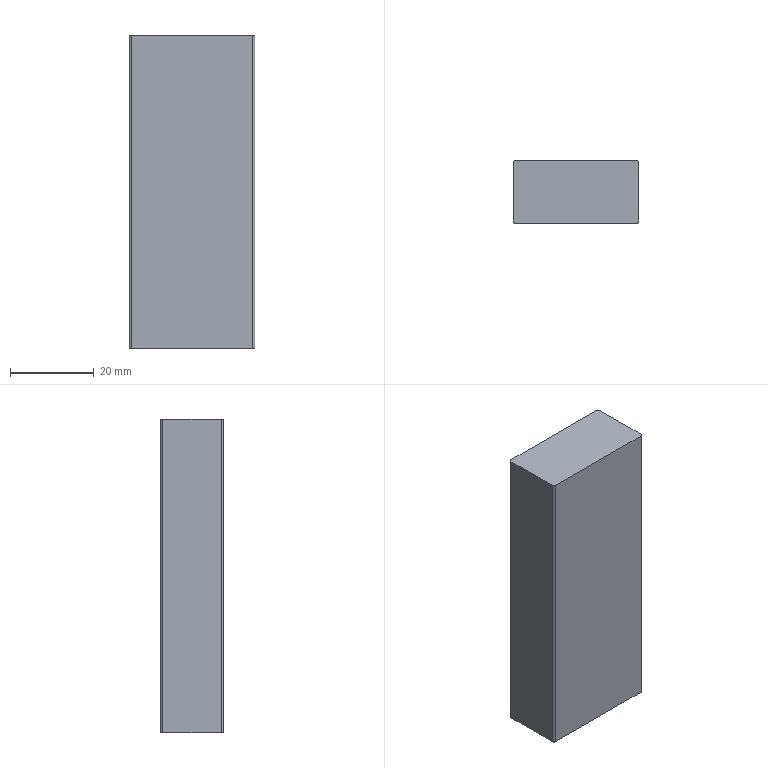Part | STEP file | 1 solid | 81 faces | box 30 x 15 x 75 mm | volume 32986 mm3 | plane 57 | other 17 | cylinder 5 | cone 2 | commonest cylinder face diameters 1 x4 5 x1